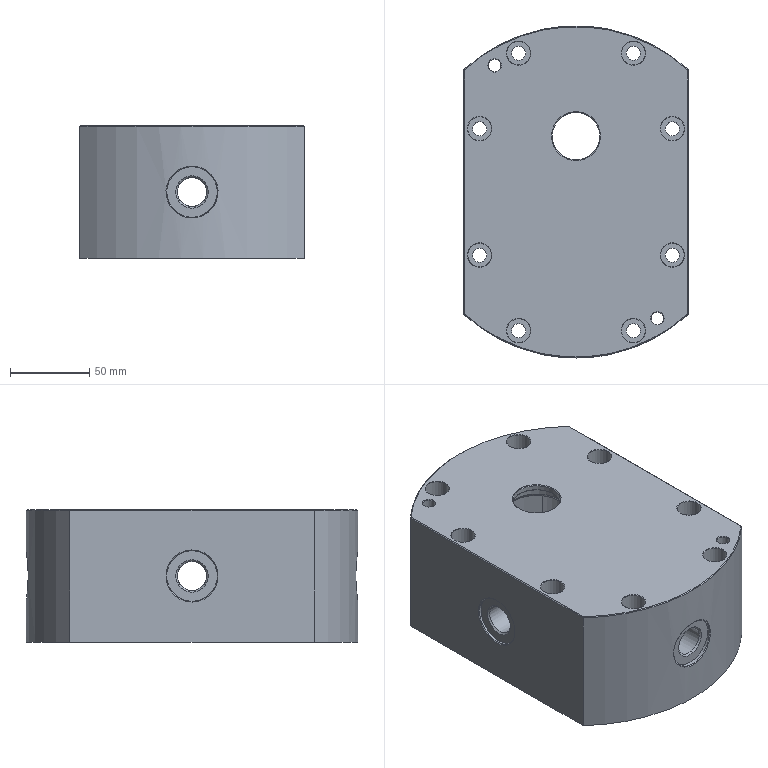NC program | NX | posted with a generic post | part box 142 x 210 x 84 mm
Lines 962 to 2056 of 7150:
(FLOOR_WALL_1 , TOOL : D25R0.5)
N1886 T05 M6
N1888 G54
N1890 G17 G0 G90 X-2.934 Y1.4 B0. C0. S2000 M3
N1892 G43 Z30. H5
N1894 Z1.5
N1896 G94 G1 X-35.372 Z0.651 F1000.
N1898 X-35.406 Y0.559 Z0.629
N1900 Y-0.559 Z0.599
N1902 X-35.372 Y-1.4 Z0.577
N1904 X0. Z-0.349
N1906 X35.372 F2200.
N1908 G3 X35.372 Y1.4 R35.4
N1910 G1 X-35.372
N1912 G3 X-35.372 Y-1.4 R35.4
N1914 G1 X0.
N1916 Y-18.9
N1918 X49.409
N1920 G3 X49.409 Y18.9 R52.9
N1922 G1 X-49.409
N1924 G3 X-49.409 Y-18.9 R52.9
N1926 G1 X0.
N1928 Y-36.4
N1930 X58.89
N1932 G3 X60.968 Y-35.2 R2.4
N1934 X60.968 Y35.2 R70.4
N1936 X58.89 Y36.4 R2.4
N1938 G1 X-58.89
N1940 G3 X-60.968 Y35.2 R2.4
N1942 X-60.968 Y-35.2 R70.4
N1944 X-58.89 Y-36.4 R2.4
N1946 G1 X0.
N1948 Z1.151
N1950 G0 X-2.934 Y1.4
N1952 G1 X-35.372 Z0.302 F1000.
N1954 X-35.406 Y0.559 Z0.28
N1956 Y-0.559 Z0.25
N1958 X-35.372 Y-1.4 Z0.228
N1960 X0. Z-0.698
N1962 X35.372 F2200.
N1964 G3 X35.372 Y1.4 R35.4
N1966 G1 X-35.372
N1968 G3 X-35.372 Y-1.4 R35.4
N1970 G1 X0.
N1972 Y-18.9
N1974 X49.409
N1976 G3 X49.409 Y18.9 R52.9
N1978 G1 X-49.409
N1980 G3 X-49.409 Y-18.9 R52.9
N1982 G1 X0.
N1984 Y-36.4
N1986 X58.89
N1988 G3 X60.968 Y-35.2 R2.4
N1990 X60.968 Y35.2 R70.4
N1992 X58.89 Y36.4 R2.4
N1994 G1 X-58.89
N1996 G3 X-60.968 Y35.2 R2.4
N1998 X-60.968 Y-35.2 R70.4
N2000 X-58.89 Y-36.4 R2.4
N2002 G1 X0.
N2004 Z0.802
N2006 G0 X-2.934 Y1.4
N2008 G1 X-35.372 Z-0.047 F1000.
N2010 X-35.406 Y0.559 Z-0.07
N2012 Y-0.559 Z-0.099
N2014 X-35.372 Y-1.4 Z-0.121
N2016 X0. Z-1.047
N2018 X35.372 F2200.
N2020 G3 X35.372 Y1.4 R35.4
N2022 G1 X-35.372
N2024 G3 X-35.372 Y-1.4 R35.4
N2026 G1 X0.
N2028 Y-18.9
N2030 X49.409
N2032 G3 X49.409 Y18.9 R52.9
N2034 G1 X-49.409
N2036 G3 X-49.409 Y-18.9 R52.9
N2038 G1 X0.
N2040 Y-36.4
N2042 X58.89
N2044 G3 X60.968 Y-35.2 R2.4
N2046 X60.968 Y35.2 R70.4
N2048 X58.89 Y36.4 R2.4
N2050 G1 X-58.89
N2052 G3 X-60.968 Y35.2 R2.4
N2054 X-60.968 Y-35.2 R70.4
N2056 X-58.89 Y-36.4 R2.4
N2058 G1 X0.
N2060 Z0.453
N2062 G0 X-2.934 Y1.4
N2064 G1 X-35.372 Z-0.397 F1000.
N2066 X-35.406 Y0.559 Z-0.419
N2068 Y-0.559 Z-0.448
N2070 X-35.372 Y-1.4 Z-0.47
N2072 X0. Z-1.396
N2074 X35.372 F2200.
N2076 G3 X35.372 Y1.4 R35.4
N2078 G1 X-35.372
N2080 G3 X-35.372 Y-1.4 R35.4
N2082 G1 X0.
N2084 Y-18.9
N2086 X49.409
N2088 G3 X49.409 Y18.9 R52.9
N2090 G1 X-49.409
N2092 G3 X-49.409 Y-18.9 R52.9
N2094 G1 X0.
N2096 Y-36.4
N2098 X58.89
N2100 G3 X60.968 Y-35.2 R2.4
N2102 X60.968 Y35.2 R70.4
N2104 X58.89 Y36.4 R2.4
N2106 G1 X-58.89
N2108 G3 X-60.968 Y35.2 R2.4
N2110 X-60.968 Y-35.2 R70.4
N2112 X-58.89 Y-36.4 R2.4
N2114 G1 X0.
N2116 Z0.104
N2118 G0 X-2.934 Y1.4
N2120 G1 X-35.372 Z-0.746 F1000.
N2122 X-35.406 Y0.559 Z-0.768
N2124 Y-0.559 Z-0.797
N2126 X-35.372 Y-1.4 Z-0.819
N2128 X0. Z-1.745
N2130 X35.372 F2200.
N2132 G3 X35.372 Y1.4 R35.4
N2134 G1 X-35.372
N2136 G3 X-35.372 Y-1.4 R35.4
N2138 G1 X0.
N2140 Y-18.9
N2142 X49.409
N2144 G3 X49.409 Y18.9 R52.9
N2146 G1 X-49.409
N2148 G3 X-49.409 Y-18.9 R52.9
N2150 G1 X0.
N2152 Y-36.4
N2154 X58.89
N2156 G3 X60.968 Y-35.2 R2.4
N2158 X60.968 Y35.2 R70.4
N2160 X58.89 Y36.4 R2.4
N2162 G1 X-58.89
N2164 G3 X-60.968 Y35.2 R2.4
N2166 X-60.968 Y-35.2 R70.4
N2168 X-58.89 Y-36.4 R2.4
N2170 G1 X0.
N2172 Z-0.245
N2174 G0 X-2.934 Y1.4
N2176 G1 X-35.372 Z-1.095 F1000.
N2178 X-35.406 Y0.559 Z-1.117
N2180 Y-0.559 Z-1.146
N2182 X-35.372 Y-1.4 Z-1.168
N2184 X0. Z-2.094
N2186 X35.372 F2200.
N2188 G3 X35.372 Y1.4 R35.4
N2190 G1 X-35.372
N2192 G3 X-35.372 Y-1.4 R35.4
N2194 G1 X0.
N2196 Y-18.9
N2198 X49.409
N2200 G3 X49.409 Y18.9 R52.9
N2202 G1 X-49.409
N2204 G3 X-49.409 Y-18.9 R52.9
N2206 G1 X0.
N2208 Y-36.4
N2210 X58.89
N2212 G3 X60.968 Y-35.2 R2.4
N2214 X60.968 Y35.2 R70.4
N2216 X58.89 Y36.4 R2.4
N2218 G1 X-58.89
N2220 G3 X-60.968 Y35.2 R2.4
N2222 X-60.968 Y-35.2 R70.4
N2224 X-58.89 Y-36.4 R2.4
N2226 G1 X0.
N2228 Z-0.594
N2230 G0 X-2.934 Y1.4
N2232 G1 X-35.372 Z-1.444 F1000.
N2234 X-35.406 Y0.559 Z-1.466
N2236 Y-0.559 Z-1.495
N2238 X-35.372 Y-1.4 Z-1.517
N2240 X0. Z-2.443
N2242 X35.372 F2200.
N2244 G3 X35.372 Y1.4 R35.4
N2246 G1 X-35.372
N2248 G3 X-35.372 Y-1.4 R35.4
N2250 G1 X0.
N2252 Y-18.9
N2254 X49.409
N2256 G3 X49.409 Y18.9 R52.9
N2258 G1 X-49.409
N2260 G3 X-49.409 Y-18.9 R52.9
N2262 G1 X0.
N2264 Y-36.4
N2266 X58.89
N2268 G3 X60.968 Y-35.2 R2.4
N2270 X60.968 Y35.2 R70.4
N2272 X58.89 Y36.4 R2.4
N2274 G1 X-58.89
N2276 G3 X-60.968 Y35.2 R2.4
N2278 X-60.968 Y-35.2 R70.4
N2280 X-58.89 Y-36.4 R2.4
N2282 G1 X0.
N2284 Z-0.943
N2286 G0 X-2.934 Y1.4
N2288 G1 X-35.372 Z-1.793 F1000.
N2290 X-35.406 Y0.559 Z-1.815
N2292 Y-0.559 Z-1.844
N2294 X-35.372 Y-1.4 Z-1.866
N2296 X0. Z-2.792
N2298 X35.372 F2200.
N2300 G3 X35.372 Y1.4 R35.4
N2302 G1 X-35.372
N2304 G3 X-35.372 Y-1.4 R35.4
N2306 G1 X0.
N2308 Y-18.9
N2310 X49.409
N2312 G3 X49.409 Y18.9 R52.9
N2314 G1 X-49.409
N2316 G3 X-49.409 Y-18.9 R52.9
N2318 G1 X0.
N2320 Y-36.4
N2322 X58.89
N2324 G3 X60.968 Y-35.2 R2.4
N2326 X60.968 Y35.2 R70.4
N2328 X58.89 Y36.4 R2.4
N2330 G1 X-58.89
N2332 G3 X-60.968 Y35.2 R2.4
N2334 X-60.968 Y-35.2 R70.4
N2336 X-58.89 Y-36.4 R2.4
N2338 G1 X0.
N2340 Z-1.292
N2342 G0 X-2.934 Y1.4
N2344 G1 X-35.372 Z-2.142 F1000.
N2346 X-35.406 Y0.559 Z-2.164
N2348 Y-0.559 Z-2.193
N2350 X-35.372 Y-1.4 Z-2.215
N2352 X0. Z-3.141
N2354 X35.372 F2200.
N2356 G3 X35.372 Y1.4 R35.4
N2358 G1 X-35.372
N2360 G3 X-35.372 Y-1.4 R35.4
N2362 G1 X0.
N2364 Y-18.9
N2366 X49.409
N2368 G3 X49.409 Y18.9 R52.9
N2370 G1 X-49.409
N2372 G3 X-49.409 Y-18.9 R52.9
N2374 G1 X0.
N2376 Y-36.4
N2378 X58.89
N2380 G3 X60.968 Y-35.2 R2.4
N2382 X60.968 Y35.2 R70.4
N2384 X58.89 Y36.4 R2.4
N2386 G1 X-58.89
N2388 G3 X-60.968 Y35.2 R2.4
N2390 X-60.968 Y-35.2 R70.4
N2392 X-58.89 Y-36.4 R2.4
N2394 G1 X0.
N2396 Z-1.641
N2398 G0 X-2.934 Y1.4
N2400 G1 X-35.372 Z-2.491 F1000.
N2402 X-35.406 Y0.559 Z-2.513
N2404 Y-0.559 Z-2.542
N2406 X-35.372 Y-1.4 Z-2.564
N2408 X0. Z-3.49
N2410 X35.372 F2200.
N2412 G3 X35.372 Y1.4 R35.4
N2414 G1 X-35.372
N2416 G3 X-35.372 Y-1.4 R35.4
N2418 G1 X0.
N2420 Y-18.9
N2422 X49.409
N2424 G3 X49.409 Y18.9 R52.9
N2426 G1 X-49.409
N2428 G3 X-49.409 Y-18.9 R52.9
N2430 G1 X0.
N2432 Y-36.4
N2434 X58.89
N2436 G3 X60.968 Y-35.2 R2.4
N2438 X60.968 Y35.2 R70.4
N2440 X58.89 Y36.4 R2.4
N2442 G1 X-58.89
N2444 G3 X-60.968 Y35.2 R2.4
N2446 X-60.968 Y-35.2 R70.4
N2448 X-58.89 Y-36.4 R2.4
N2450 G1 X0.
N2452 Z-1.99
N2454 G0 X-2.934 Y1.4
N2456 G1 X-35.372 Z-2.84 F1000.
N2458 X-35.406 Y0.559 Z-2.862
N2460 Y-0.559 Z-2.891
N2462 X-35.372 Y-1.4 Z-2.913
N2464 X0. Z-3.839
N2466 X35.372 F2200.
N2468 G3 X35.372 Y1.4 R35.4
N2470 G1 X-35.372
N2472 G3 X-35.372 Y-1.4 R35.4
N2474 G1 X0.
N2476 Y-18.9
N2478 X49.409
N2480 G3 X49.409 Y18.9 R52.9
N2482 G1 X-49.409
N2484 G3 X-49.409 Y-18.9 R52.9
N2486 G1 X0.
N2488 Y-36.4
N2490 X58.89
N2492 G3 X60.968 Y-35.2 R2.4
N2494 X60.968 Y35.2 R70.4
N2496 X58.89 Y36.4 R2.4
N2498 G1 X-58.89
N2500 G3 X-60.968 Y35.2 R2.4
N2502 X-60.968 Y-35.2 R70.4
N2504 X-58.89 Y-36.4 R2.4
N2506 G1 X0.
N2508 Z-2.339
N2510 G0 X-2.934 Y1.4
N2512 G1 X-35.372 Z-3.189 F1000.
N2514 X-35.406 Y0.559 Z-3.211
N2516 Y-0.559 Z-3.24
N2518 X-35.372 Y-1.4 Z-3.262
N2520 X0. Z-4.188
N2522 X35.372 F2200.
N2524 G3 X35.372 Y1.4 R35.4
N2526 G1 X-35.372
N2528 G3 X-35.372 Y-1.4 R35.4
N2530 G1 X0.
N2532 Y-18.9
N2534 X49.409
N2536 G3 X49.409 Y18.9 R52.9
N2538 G1 X-49.409
N2540 G3 X-49.409 Y-18.9 R52.9
N2542 G1 X0.
N2544 Y-36.4
N2546 X58.89
N2548 G3 X60.968 Y-35.2 R2.4
N2550 X60.968 Y35.2 R70.4
N2552 X58.89 Y36.4 R2.4
N2554 G1 X-58.89
N2556 G3 X-60.968 Y35.2 R2.4
N2558 X-60.968 Y-35.2 R70.4
N2560 X-58.89 Y-36.4 R2.4
N2562 G1 X0.
N2564 Z-2.688
N2566 G0 X-2.934 Y1.4
N2568 G1 X-35.372 Z-3.538 F1000.
N2570 X-35.406 Y0.559 Z-3.56
N2572 Y-0.559 Z-3.589
N2574 X-35.372 Y-1.4 Z-3.611
N2576 X0. Z-4.537
N2578 X35.372 F2200.
N2580 G3 X35.372 Y1.4 R35.4
N2582 G1 X-35.372
N2584 G3 X-35.372 Y-1.4 R35.4
N2586 G1 X0.
N2588 Y-18.9
N2590 X49.409
N2592 G3 X49.409 Y18.9 R52.9
N2594 G1 X-49.409
N2596 G3 X-49.409 Y-18.9 R52.9
N2598 G1 X0.
N2600 Y-36.4
N2602 X58.89
N2604 G3 X60.968 Y-35.2 R2.4
N2606 X60.968 Y35.2 R70.4
N2608 X58.89 Y36.4 R2.4
N2610 G1 X-58.89
N2612 G3 X-60.968 Y35.2 R2.4
N2614 X-60.968 Y-35.2 R70.4
N2616 X-58.89 Y-36.4 R2.4
N2618 G1 X0.
N2620 Z-3.037
N2622 G0 X-2.934 Y1.4
N2624 G1 X-35.372 Z-3.887 F1000.
N2626 X-35.406 Y0.559 Z-3.909
N2628 Y-0.559 Z-3.938
N2630 X-35.372 Y-1.4 Z-3.96
N2632 X0. Z-4.886
N2634 X35.372 F2200.
N2636 G3 X35.372 Y1.4 R35.4
N2638 G1 X-35.372
N2640 G3 X-35.372 Y-1.4 R35.4
N2642 G1 X0.
N2644 Y-18.9
N2646 X49.409
N2648 G3 X49.409 Y18.9 R52.9
N2650 G1 X-49.409
N2652 G3 X-49.409 Y-18.9 R52.9
N2654 G1 X0.
N2656 Y-36.4
N2658 X58.89
N2660 G3 X60.968 Y-35.2 R2.4
N2662 X60.968 Y35.2 R70.4
N2664 X58.89 Y36.4 R2.4
N2666 G1 X-58.89
N2668 G3 X-60.968 Y35.2 R2.4
N2670 X-60.968 Y-35.2 R70.4
N2672 X-58.89 Y-36.4 R2.4
N2674 G1 X0.
N2676 Z-3.386
N2678 G0 X-2.934 Y1.4
N2680 G1 X-35.372 Z-4.236 F1000.
N2682 X-35.406 Y0.559 Z-4.258
N2684 Y-0.559 Z-4.287
N2686 X-35.372 Y-1.4 Z-4.309
N2688 X0. Z-5.235
N2690 X35.372 F2200.
N2692 G3 X35.372 Y1.4 R35.4
N2694 G1 X-35.372
N2696 G3 X-35.372 Y-1.4 R35.4
N2698 G1 X0.
N2700 Y-18.9
N2702 X49.409
N2704 G3 X49.409 Y18.9 R52.9
N2706 G1 X-49.409
N2708 G3 X-49.409 Y-18.9 R52.9
N2710 G1 X0.
N2712 Y-36.4
N2714 X58.89
N2716 G3 X60.968 Y-35.2 R2.4
N2718 X60.968 Y35.2 R70.4
N2720 X58.89 Y36.4 R2.4
N2722 G1 X-58.89
N2724 G3 X-60.968 Y35.2 R2.4
N2726 X-60.968 Y-35.2 R70.4
N2728 X-58.89 Y-36.4 R2.4
N2730 G1 X0.
N2732 Z-3.735
N2734 G0 X-2.934 Y1.4
N2736 G1 X-35.372 Z-4.585 F1000.
N2738 X-35.406 Y0.559 Z-4.607
N2740 Y-0.559 Z-4.636
N2742 X-35.372 Y-1.4 Z-4.658
N2744 X0. Z-5.584
N2746 X35.372 F2200.
N2748 G3 X35.372 Y1.4 R35.4
N2750 G1 X-35.372
N2752 G3 X-35.372 Y-1.4 R35.4
N2754 G1 X0.
N2756 Y-18.9
N2758 X49.409
N2760 G3 X49.409 Y18.9 R52.9
N2762 G1 X-49.409
N2764 G3 X-49.409 Y-18.9 R52.9
N2766 G1 X0.
N2768 Y-36.4
N2770 X58.89
N2772 G3 X60.968 Y-35.2 R2.4
N2774 X60.968 Y35.2 R70.4
N2776 X58.89 Y36.4 R2.4
N2778 G1 X-58.89
N2780 G3 X-60.968 Y35.2 R2.4
N2782 X-60.968 Y-35.2 R70.4
N2784 X-58.89 Y-36.4 R2.4
N2786 G1 X0.
N2788 Z-4.084
N2790 G0 X-2.934 Y1.4
N2792 G1 X-35.372 Z-4.934 F1000.
N2794 X-35.406 Y0.559 Z-4.956
N2796 Y-0.559 Z-4.985
N2798 X-35.372 Y-1.4 Z-5.007
N2800 X0. Z-5.933
N2802 X35.372 F2200.
N2804 G3 X35.372 Y1.4 R35.4
N2806 G1 X-35.372
N2808 G3 X-35.372 Y-1.4 R35.4
N2810 G1 X0.
N2812 Y-18.9
N2814 X49.409
N2816 G3 X49.409 Y18.9 R52.9
N2818 G1 X-49.409
N2820 G3 X-49.409 Y-18.9 R52.9
N2822 G1 X0.
N2824 Y-36.4
N2826 X58.89
N2828 G3 X60.968 Y-35.2 R2.4
N2830 X60.968 Y35.2 R70.4
N2832 X58.89 Y36.4 R2.4
N2834 G1 X-58.89
N2836 G3 X-60.968 Y35.2 R2.4
N2838 X-60.968 Y-35.2 R70.4
N2840 X-58.89 Y-36.4 R2.4
N2842 G1 X0.
N2844 Z-4.433
N2846 G0 X-2.934 Y1.4
N2848 G1 X-35.372 Z-5.283 F1000.
N2850 X-35.406 Y0.559 Z-5.305
N2852 Y-0.559 Z-5.334
N2854 X-35.372 Y-1.4 Z-5.356
N2856 X0. Z-6.283
N2858 X35.372 F2200.
N2860 G3 X35.372 Y1.4 R35.4
N2862 G1 X-35.372
N2864 G3 X-35.372 Y-1.4 R35.4
N2866 G1 X0.
N2868 Y-18.9
N2870 X49.409
N2872 G3 X49.409 Y18.9 R52.9
N2874 G1 X-49.409
N2876 G3 X-49.409 Y-18.9 R52.9
N2878 G1 X0.
N2880 Y-36.4
N2882 X58.89
N2884 G3 X60.968 Y-35.2 R2.4
N2886 X60.968 Y35.2 R70.4
N2888 X58.89 Y36.4 R2.4
N2890 G1 X-58.89
N2892 G3 X-60.968 Y35.2 R2.4
N2894 X-60.968 Y-35.2 R70.4
N2896 X-58.89 Y-36.4 R2.4
N2898 G1 X0.
N2900 Z-4.783
N2902 G0 X-2.934 Y1.4
N2904 G1 X-35.372 Z-5.632 F1000.
N2906 X-35.406 Y0.559 Z-5.654
N2908 Y-0.559 Z-5.683
N2910 X-35.372 Y-1.4 Z-5.705
N2912 X0. Z-6.632
N2914 X35.372 F2200.
N2916 G3 X35.372 Y1.4 R35.4
N2918 G1 X-35.372
N2920 G3 X-35.372 Y-1.4 R35.4
N2922 G1 X0.
N2924 Y-18.9
N2926 X49.409
N2928 G3 X49.409 Y18.9 R52.9
N2930 G1 X-49.409
N2932 G3 X-49.409 Y-18.9 R52.9
N2934 G1 X0.
N2936 Y-36.4
N2938 X58.89
N2940 G3 X60.968 Y-35.2 R2.4
N2942 X60.968 Y35.2 R70.4
N2944 X58.89 Y36.4 R2.4
N2946 G1 X-58.89
N2948 G3 X-60.968 Y35.2 R2.4
N2950 X-60.968 Y-35.2 R70.4
N2952 X-58.89 Y-36.4 R2.4
N2954 G1 X0.
N2956 Z-5.132
N2958 G0 X-2.934 Y1.4
N2960 G1 X-35.372 Z-5.981 F1000.
N2962 X-35.406 Y0.559 Z-6.003
N2964 Y-0.559 Z-6.032
N2966 X-35.372 Y-1.4 Z-6.054
N2968 X0. Z-6.981
N2970 X35.372 F2200.
N2972 G3 X35.372 Y1.4 R35.4
N2974 G1 X-35.372
N2976 G3 X-35.372 Y-1.4 R35.4
N2978 G1 X0.
N2980 Y-18.9
N2982 X49.409
N2984 G3 X49.409 Y18.9 R52.9
N2986 G1 X-49.409
N2988 G3 X-49.409 Y-18.9 R52.9
N2990 G1 X0.
N2992 Y-36.4
N2994 X58.89
N2996 G3 X60.968 Y-35.2 R2.4
N2998 X60.968 Y35.2 R70.4
N3000 X58.89 Y36.4 R2.4
N3002 G1 X-58.89
N3004 G3 X-60.968 Y35.2 R2.4
N3006 X-60.968 Y-35.2 R70.4
N3008 X-58.89 Y-36.4 R2.4
N3010 G1 X0.
N3012 Z-5.481
N3014 G0 X-2.934 Y1.4
N3016 G1 X-35.372 Z-6.33 F1000.
N3018 X-35.406 Y0.559 Z-6.352
N3020 Y-0.559 Z-6.381
N3022 X-35.372 Y-1.4 Z-6.403
N3024 X0. Z-7.33
N3026 X35.372 F2200.
N3028 G3 X35.372 Y1.4 R35.4
N3030 G1 X-35.372
N3032 G3 X-35.372 Y-1.4 R35.4
N3034 G1 X0.
N3036 Y-18.9
N3038 X49.409
N3040 G3 X49.409 Y18.9 R52.9
N3042 G1 X-49.409
N3044 G3 X-49.409 Y-18.9 R52.9
N3046 G1 X0.
N3048 Y-36.4
N3050 X58.89
N3052 G3 X60.968 Y-35.2 R2.4
N3054 X60.968 Y35.2 R70.4
N3056 X58.89 Y36.4 R2.4
N3058 G1 X-58.89
N3060 G3 X-60.968 Y35.2 R2.4
N3062 X-60.968 Y-35.2 R70.4
N3064 X-58.89 Y-36.4 R2.4
N3066 G1 X0.
N3068 Z-5.83
N3070 G0 X-2.934 Y1.4
N3072 G1 X-35.372 Z-6.679 F1000.
N3074 X-35.406 Y0.559 Z-6.701
N3076 Y-0.559 Z-6.73
N3078 X-35.372 Y-1.4 Z-6.752
N3080 X0. Z-7.679
N3082 X35.372 F2200.
N3084 G3 X35.372 Y1.4 R35.4
N3086 G1 X-35.372
N3088 G3 X-35.372 Y-1.4 R35.4
N3090 G1 X0.
N3092 Y-18.9
N3094 X49.409
N3096 G3 X49.409 Y18.9 R52.9
N3098 G1 X-49.409
N3100 G3 X-49.409 Y-18.9 R52.9
N3102 G1 X0.
N3104 Y-36.4
N3106 X58.89
N3108 G3 X60.968 Y-35.2 R2.4
N3110 X60.968 Y35.2 R70.4
N3112 X58.89 Y36.4 R2.4
N3114 G1 X-58.89
N3116 G3 X-60.968 Y35.2 R2.4
N3118 X-60.968 Y-35.2 R70.4
N3120 X-58.89 Y-36.4 R2.4
N3122 G1 X0.
N3124 Z-6.179
N3126 G0 X-2.934 Y1.4
N3128 G1 X-35.372 Z-7.028 F1000.
N3130 X-35.406 Y0.559 Z-7.05
N3132 Y-0.559 Z-7.079
N3134 X-35.372 Y-1.4 Z-7.101
N3136 X0. Z-8.028
N3138 X35.372 F2200.
N3140 G3 X35.372 Y1.4 R35.4
N3142 G1 X-35.372
N3144 G3 X-35.372 Y-1.4 R35.4
N3146 G1 X0.
N3148 Y-18.9
N3150 X49.409
N3152 G3 X49.409 Y18.9 R52.9
N3154 G1 X-49.409
N3156 G3 X-49.409 Y-18.9 R52.9
N3158 G1 X0.
N3160 Y-36.4
N3162 X58.89
N3164 G3 X60.968 Y-35.2 R2.4
N3166 X60.968 Y35.2 R70.4
N3168 X58.89 Y36.4 R2.4
N3170 G1 X-58.89
N3172 G3 X-60.968 Y35.2 R2.4
N3174 X-60.968 Y-35.2 R70.4
N3176 X-58.89 Y-36.4 R2.4
N3178 G1 X0.
N3180 Z-6.528
N3182 G0 X-2.934 Y1.4
N3184 G1 X-35.372 Z-7.377 F1000.
N3186 X-35.406 Y0.559 Z-7.399
N3188 Y-0.559 Z-7.428
N3190 X-35.372 Y-1.4 Z-7.45
N3192 X0. Z-8.377
N3194 X35.372 F2200.
N3196 G3 X35.372 Y1.4 R35.4
N3198 G1 X-35.372
N3200 G3 X-35.372 Y-1.4 R35.4
N3202 G1 X0.
N3204 Y-18.9
N3206 X49.409
N3208 G3 X49.409 Y18.9 R52.9
N3210 G1 X-49.409
N3212 G3 X-49.409 Y-18.9 R52.9
N3214 G1 X0.
N3216 Y-36.4
N3218 X58.89
N3220 G3 X60.968 Y-35.2 R2.4
N3222 X60.968 Y35.2 R70.4
N3224 X58.89 Y36.4 R2.4
N3226 G1 X-58.89
N3228 G3 X-60.968 Y35.2 R2.4
N3230 X-60.968 Y-35.2 R70.4
N3232 X-58.89 Y-36.4 R2.4
N3234 G1 X0.
N3236 Z-6.877
N3238 G0 X-2.934 Y1.4
N3240 G1 X-35.372 Z-7.726 F1000.
N3242 X-35.406 Y0.559 Z-7.748
N3244 Y-0.559 Z-7.777
N3246 X-35.372 Y-1.4 Z-7.799
N3248 X0. Z-8.726
N3250 X35.372 F2200.
N3252 G3 X35.372 Y1.4 R35.4
N3254 G1 X-35.372
N3256 G3 X-35.372 Y-1.4 R35.4
N3258 G1 X0.
N3260 Y-18.9
N3262 X49.409
N3264 G3 X49.409 Y18.9 R52.9
N3266 G1 X-49.409
N3268 G3 X-49.409 Y-18.9 R52.9
N3270 G1 X0.
N3272 Y-36.4
N3274 X58.89
N3276 G3 X60.968 Y-35.2 R2.4
N3278 X60.968 Y35.2 R70.4
N3280 X58.89 Y36.4 R2.4
N3282 G1 X-58.89
N3284 G3 X-60.968 Y35.2 R2.4
N3286 X-60.968 Y-35.2 R70.4
N3288 X-58.89 Y-36.4 R2.4
N3290 G1 X0.
N3292 Z-7.226
N3294 G0 X-2.934 Y1.4
N3296 G1 X-35.372 Z-8.075 F1000.
N3298 X-35.406 Y0.559 Z-8.097
N3300 Y-0.559 Z-8.126
N3302 X-35.372 Y-1.4 Z-8.149
N3304 X0. Z-9.075
N3306 X35.372 F2200.
N3308 G3 X35.372 Y1.4 R35.4
N3310 G1 X-35.372
N3312 G3 X-35.372 Y-1.4 R35.4
N3314 G1 X0.
N3316 Y-18.9
N3318 X49.409
N3320 G3 X49.409 Y18.9 R52.9
N3322 G1 X-49.409
N3324 G3 X-49.409 Y-18.9 R52.9
N3326 G1 X0.
N3328 Y-36.4
N3330 X58.89
N3332 G3 X60.968 Y-35.2 R2.4
N3334 X60.968 Y35.2 R70.4
N3336 X58.89 Y36.4 R2.4
N3338 G1 X-58.89
N3340 G3 X-60.968 Y35.2 R2.4
N3342 X-60.968 Y-35.2 R70.4
N3344 X-58.89 Y-36.4 R2.4
N3346 G1 X0.
N3348 Z-7.575
N3350 G0 X-2.934 Y1.4
N3352 G1 X-35.372 Z-8.424 F1000.
N3354 X-35.406 Y0.559 Z-8.446
N3356 Y-0.559 Z-8.475
N3358 X-35.372 Y-1.4 Z-8.498
N3360 X0. Z-9.424
N3362 X35.372 F2200.
N3364 G3 X35.372 Y1.4 R35.4
N3366 G1 X-35.372
N3368 G3 X-35.372 Y-1.4 R35.4
N3370 G1 X0.
N3372 Y-18.9
N3374 X49.409
N3376 G3 X49.409 Y18.9 R52.9
N3378 G1 X-49.409
N3380 G3 X-49.409 Y-18.9 R52.9
N3382 G1 X0.
N3384 Y-36.4
N3386 X58.89
N3388 G3 X60.968 Y-35.2 R2.4
N3390 X60.968 Y35.2 R70.4
N3392 X58.89 Y36.4 R2.4
N3394 G1 X-58.89
N3396 G3 X-60.968 Y35.2 R2.4
N3398 X-60.968 Y-35.2 R70.4
N3400 X-58.89 Y-36.4 R2.4
N3402 G1 X0.
N3404 Z-7.924
N3406 G0 X-2.934 Y1.4
N3408 G1 X-35.372 Z-8.773 F1000.
N3410 X-35.406 Y0.559 Z-8.795
N3412 Y-0.559 Z-8.825
N3414 X-35.372 Y-1.4 Z-8.847
N3416 X0. Z-9.773
N3418 X35.372 F2200.
N3420 G3 X35.372 Y1.4 R35.4
N3422 G1 X-35.372
N3424 G3 X-35.372 Y-1.4 R35.4
N3426 G1 X0.
N3428 Y-18.9
N3430 X49.409
N3432 G3 X49.409 Y18.9 R52.9
N3434 G1 X-49.409
N3436 G3 X-49.409 Y-18.9 R52.9
N3438 G1 X0.
N3440 Y-36.4
N3442 X58.89
N3444 G3 X60.968 Y-35.2 R2.4
N3446 X60.968 Y35.2 R70.4
N3448 X58.89 Y36.4 R2.4
N3450 G1 X-58.89
N3452 G3 X-60.968 Y35.2 R2.4
N3454 X-60.968 Y-35.2 R70.4
N3456 X-58.89 Y-36.4 R2.4
N3458 G1 X0.
N3460 Z-8.273
N3462 G0 X-2.934 Y1.4
N3464 G1 X-35.372 Z-9.122 F1000.
N3466 X-35.406 Y0.559 Z-9.144
N3468 Y-0.559 Z-9.174
N3470 X-35.372 Y-1.4 Z-9.196
N3472 X0. Z-10.122
N3474 X35.372 F2200.
N3476 G3 X35.372 Y1.4 R35.4
N3478 G1 X-35.372
N3480 G3 X-35.372 Y-1.4 R35.4
N3482 G1 X0.
N3484 Y-18.9
N3486 X49.409
N3488 G3 X49.409 Y18.9 R52.9
N3490 G1 X-49.409
N3492 G3 X-49.409 Y-18.9 R52.9
N3494 G1 X0.
N3496 Y-36.4
N3498 X58.89
N3500 G3 X60.968 Y-35.2 R2.4
N3502 X60.968 Y35.2 R70.4
N3504 X58.89 Y36.4 R2.4
N3506 G1 X-58.89
N3508 G3 X-60.968 Y35.2 R2.4
N3510 X-60.968 Y-35.2 R70.4
N3512 X-58.89 Y-36.4 R2.4
N3514 G1 X0.
N3516 Z-8.622
N3518 G0 X-2.934 Y1.4
N3520 G1 X-35.372 Z-9.471 F1000.
N3522 X-35.406 Y0.559 Z-9.493
N3524 Y-0.559 Z-9.523
N3526 X-35.372 Y-1.4 Z-9.545
N3528 X0. Z-10.471
N3530 X35.372 F2200.
N3532 G3 X35.372 Y1.4 R35.4
N3534 G1 X-35.372
N3536 G3 X-35.372 Y-1.4 R35.4
N3538 G1 X0.
N3540 Y-18.9
N3542 X49.409
N3544 G3 X49.409 Y18.9 R52.9
N3546 G1 X-49.409
N3548 G3 X-49.409 Y-18.9 R52.9
N3550 G1 X0.
N3552 Y-36.4
N3554 X58.89
N3556 G3 X60.968 Y-35.2 R2.4
N3558 X60.968 Y35.2 R70.4
N3560 X58.89 Y36.4 R2.4
N3562 G1 X-58.89
N3564 G3 X-60.968 Y35.2 R2.4
N3566 X-60.968 Y-35.2 R70.4
N3568 X-58.89 Y-36.4 R2.4
N3570 G1 X0.
N3572 Z-8.971
N3574 G0 X-2.934 Y1.4
N3576 G1 X-35.372 Z-9.82 F1000.
N3578 X-35.406 Y0.559 Z-9.842
N3580 Y-0.559 Z-9.872
N3582 X-35.372 Y-1.4 Z-9.894
N3584 X0. Z-10.82
N3586 X35.372 F2200.
N3588 G3 X35.372 Y1.4 R35.4
N3590 G1 X-35.372
N3592 G3 X-35.372 Y-1.4 R35.4
N3594 G1 X0.
N3596 Y-18.9
N3598 X49.409
N3600 G3 X49.409 Y18.9 R52.9
N3602 G1 X-49.409
N3604 G3 X-49.409 Y-18.9 R52.9
N3606 G1 X0.
N3608 Y-36.4
N3610 X58.89
N3612 G3 X60.968 Y-35.2 R2.4
N3614 X60.968 Y35.2 R70.4
N3616 X58.89 Y36.4 R2.4
N3618 G1 X-58.89
N3620 G3 X-60.968 Y35.2 R2.4
N3622 X-60.968 Y-35.2 R70.4
N3624 X-58.89 Y-36.4 R2.4
N3626 G1 X0.
N3628 Z-9.32
N3630 G0 X-2.934 Y1.4
N3632 G1 X-35.372 Z-10.169 F1000.
N3634 X-35.406 Y0.559 Z-10.191
N3636 Y-0.559 Z-10.221
N3638 X-35.372 Y-1.4 Z-10.243
N3640 X0. Z-11.169
N3642 X35.372 F2200.
N3644 G3 X35.372 Y1.4 R35.4
N3646 G1 X-35.372
N3648 G3 X-35.372 Y-1.4 R35.4
N3650 G1 X0.
N3652 Y-18.9
N3654 X49.409
N3656 G3 X49.409 Y18.9 R52.9
N3658 G1 X-49.409
N3660 G3 X-49.409 Y-18.9 R52.9
N3662 G1 X0.
N3664 Y-36.4
N3666 X58.89
N3668 G3 X60.968 Y-35.2 R2.4
N3670 X60.968 Y35.2 R70.4
N3672 X58.89 Y36.4 R2.4
N3674 G1 X-58.89
N3676 G3 X-60.968 Y35.2 R2.4
N3678 X-60.968 Y-35.2 R70.4
N3680 X-58.89 Y-36.4 R2.4
N3682 G1 X0.
N3684 Z-9.669
N3686 G0 X-2.934 Y1.4
N3688 G1 X-35.372 Z-10.518 F1000.
N3690 X-35.406 Y0.559 Z-10.54
N3692 Y-0.559 Z-10.57
N3694 X-35.372 Y-1.4 Z-10.592
N3696 X0. Z-11.518
N3698 X35.372 F2200.
N3700 G3 X35.372 Y1.4 R35.4
N3702 G1 X-35.372
N3704 G3 X-35.372 Y-1.4 R35.4
N3706 G1 X0.
N3708 Y-18.9
N3710 X49.409
N3712 G3 X49.409 Y18.9 R52.9
N3714 G1 X-49.409
N3716 G3 X-49.409 Y-18.9 R52.9
N3718 G1 X0.
N3720 Y-36.4
N3722 X58.89
N3724 G3 X60.968 Y-35.2 R2.4
N3726 X60.968 Y35.2 R70.4
N3728 X58.89 Y36.4 R2.4
N3730 G1 X-58.89
N3732 G3 X-60.968 Y35.2 R2.4
N3734 X-60.968 Y-35.2 R70.4
N3736 X-58.89 Y-36.4 R2.4
N3738 G1 X0.
N3740 Z-10.018
N3742 G0 X-2.934 Y1.4
N3744 G1 X-35.372 Z-10.867 F1000.
N3746 X-35.406 Y0.559 Z-10.889
N3748 Y-0.559 Z-10.919
N3750 X-35.372 Y-1.4 Z-10.941
N3752 X0. Z-11.867
N3754 X35.372 F2200.
N3756 G3 X35.372 Y1.4 R35.4
N3758 G1 X-35.372
N3760 G3 X-35.372 Y-1.4 R35.4
N3762 G1 X0.
N3764 Y-18.9
N3766 X49.409
N3768 G3 X49.409 Y18.9 R52.9
N3770 G1 X-49.409
N3772 G3 X-49.409 Y-18.9 R52.9
N3774 G1 X0.
N3776 Y-36.4
N3778 X58.89
N3780 G3 X60.968 Y-35.2 R2.4
N3782 X60.968 Y35.2 R70.4
N3784 X58.89 Y36.4 R2.4
N3786 G1 X-58.89
N3788 G3 X-60.968 Y35.2 R2.4
N3790 X-60.968 Y-35.2 R70.4
N3792 X-58.89 Y-36.4 R2.4
N3794 G1 X0.
N3796 Z-10.367
N3798 G0 X-2.934 Y1.4
N3800 G1 X-35.372 Z-11.216 F1000.
N3802 X-35.406 Y0.559 Z-11.238
N3804 Y-0.559 Z-11.268
N3806 X-35.372 Y-1.4 Z-11.29
N3808 X0. Z-12.216
N3810 X35.372 F2200.
N3812 G3 X35.372 Y1.4 R35.4
N3814 G1 X-35.372
N3816 G3 X-35.372 Y-1.4 R35.4
N3818 G1 X0.
N3820 Y-18.9
N3822 X49.409
N3824 G3 X49.409 Y18.9 R52.9
N3826 G1 X-49.409
N3828 G3 X-49.409 Y-18.9 R52.9
N3830 G1 X0.
N3832 Y-36.4
N3834 X58.89
N3836 G3 X60.968 Y-35.2 R2.4
N3838 X60.968 Y35.2 R70.4
N3840 X58.89 Y36.4 R2.4
N3842 G1 X-58.89
N3844 G3 X-60.968 Y35.2 R2.4
N3846 X-60.968 Y-35.2 R70.4
N3848 X-58.89 Y-36.4 R2.4
N3850 G1 X0.
N3852 Z-10.716
N3854 G0 X-2.934 Y1.4
N3856 G1 X-35.372 Z-11.565 F1000.
N3858 X-35.406 Y0.559 Z-11.587
N3860 Y-0.559 Z-11.617
N3862 X-35.372 Y-1.4 Z-11.639
N3864 X0. Z-12.565
N3866 X35.372 F2200.
N3868 G3 X35.372 Y1.4 R35.4
N3870 G1 X-35.372
N3872 G3 X-35.372 Y-1.4 R35.4
N3874 G1 X0.
N3876 Y-18.9
N3878 X49.409
N3880 G3 X49.409 Y18.9 R52.9
N3882 G1 X-49.409
N3884 G3 X-49.409 Y-18.9 R52.9
N3886 G1 X0.
N3888 Y-36.4
N3890 X58.89
N3892 G3 X60.968 Y-35.2 R2.4
N3894 X60.968 Y35.2 R70.4
N3896 X58.89 Y36.4 R2.4
N3898 G1 X-58.89
N3900 G3 X-60.968 Y35.2 R2.4
N3902 X-60.968 Y-35.2 R70.4
N3904 X-58.89 Y-36.4 R2.4
N3906 G1 X0.
N3908 Z-11.065
N3910 G0 X-2.934 Y1.4
N3912 G1 X-35.372 Z-11.914 F1000.
N3914 X-35.406 Y0.559 Z-11.937
N3916 Y-0.559 Z-11.966
N3918 X-35.372 Y-1.4 Z-11.988
N3920 X0. Z-12.914
N3922 X35.372 F2200.
N3924 G3 X35.372 Y1.4 R35.4
N3926 G1 X-35.372
N3928 G3 X-35.372 Y-1.4 R35.4
N3930 G1 X0.
N3932 Y-18.9
N3934 X49.409
N3936 G3 X49.409 Y18.9 R52.9
N3938 G1 X-49.409
N3940 G3 X-49.409 Y-18.9 R52.9
N3942 G1 X0.
N3944 Y-36.4
N3946 X58.89
N3948 G3 X60.968 Y-35.2 R2.4
N3950 X60.968 Y35.2 R70.4
N3952 X58.89 Y36.4 R2.4
N3954 G1 X-58.89
N3956 G3 X-60.968 Y35.2 R2.4
N3958 X-60.968 Y-35.2 R70.4
N3960 X-58.89 Y-36.4 R2.4
N3962 G1 X0.
N3964 Z-11.414
N3966 G0 X-2.934 Y1.4
N3968 G1 X-35.372 Z-12.263 F1000.
N3970 X-35.406 Y0.559 Z-12.286
N3972 Y-0.559 Z-12.315
N3974 X-35.372 Y-1.4 Z-12.337
N3976 X0. Z-13.263
N3978 X35.372 F2200.
N3980 G3 X35.372 Y1.4 R35.4
N3982 G1 X-35.372
N3984 G3 X-35.372 Y-1.4 R35.4
N3986 G1 X0.
N3988 Y-18.9
N3990 X49.409
N3992 G3 X49.409 Y18.9 R52.9
N3994 G1 X-49.409
N3996 G3 X-49.409 Y-18.9 R52.9
N3998 G1 X0.
N4000 Y-36.4
N4002 X58.89
N4004 G3 X60.968 Y-35.2 R2.4
N4006 X60.968 Y35.2 R70.4
N4008 X58.89 Y36.4 R2.4
N4010 G1 X-58.89
N4012 G3 X-60.968 Y35.2 R2.4
N4014 X-60.968 Y-35.2 R70.4
N4016 X-58.89 Y-36.4 R2.4
N4018 G1 X0.
N4020 Z-11.763
N4022 G0 X-2.934 Y1.4
N4024 G1 X-35.372 Z-12.613 F1000.
N4026 X-35.406 Y0.559 Z-12.635
N4028 Y-0.559 Z-12.664
N4030 X-35.372 Y-1.4 Z-12.686
N4032 X0. Z-13.612
N4034 X35.372 F2200.
N4036 G3 X35.372 Y1.4 R35.4
N4038 G1 X-35.372
N4040 G3 X-35.372 Y-1.4 R35.4
N4042 G1 X0.
N4044 Y-18.9
N4046 X49.409
N4048 G3 X49.409 Y18.9 R52.9
N4050 G1 X-49.409
N4052 G3 X-49.409 Y-18.9 R52.9
N4054 G1 X0.
N4056 Y-36.4
N4058 X58.89
N4060 G3 X60.968 Y-35.2 R2.4
N4062 X60.968 Y35.2 R70.4
N4064 X58.89 Y36.4 R2.4
N4066 G1 X-58.89
N4068 G3 X-60.968 Y35.2 R2.4